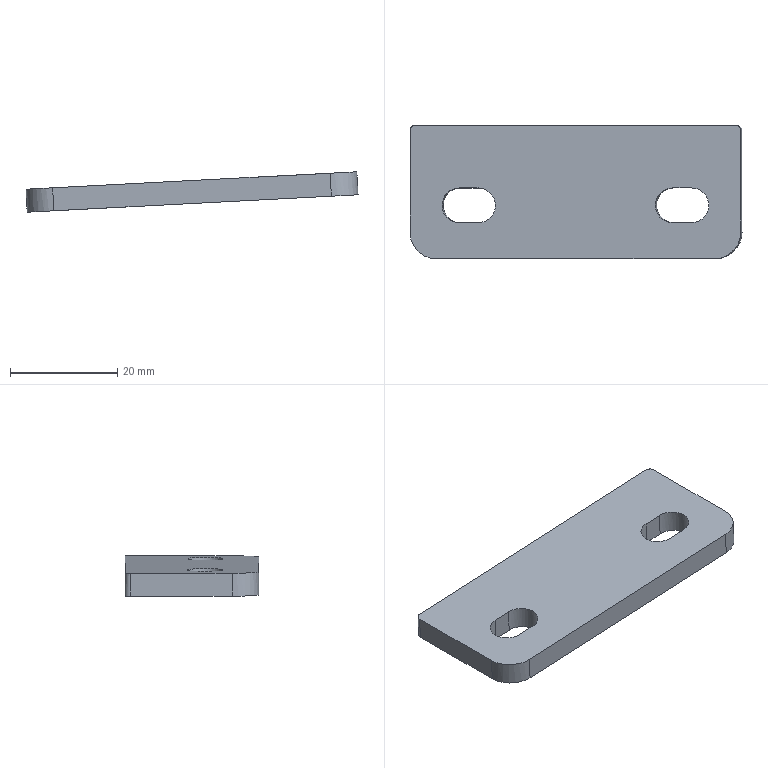Part | STEP file | PRT0001_68_25 | 1 solid | 18 faces | box 62.055 x 25 x 7.544 mm | volume 6128 mm3 | plane 10 | other 8